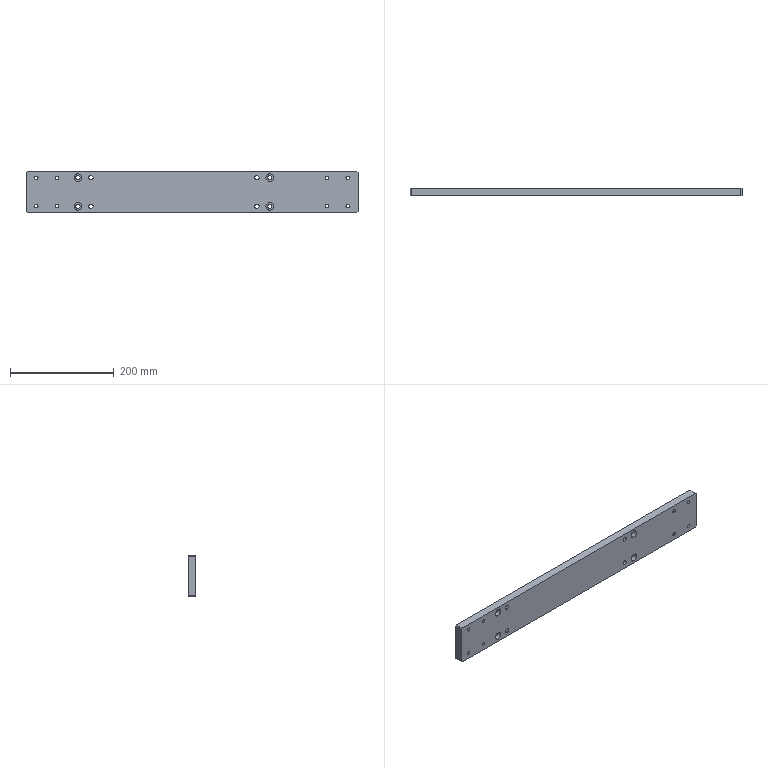Part | SolidWorks | features BaseBody 1 | 1 solid | 78 faces | box 640 x 15 x 80 mm | volume 749369 mm3 | cylinder 56 | plane 22 | commonest cylinder face diameters 6.6 x16 11 x16 8.4 x8 8.5 x8 15 x8